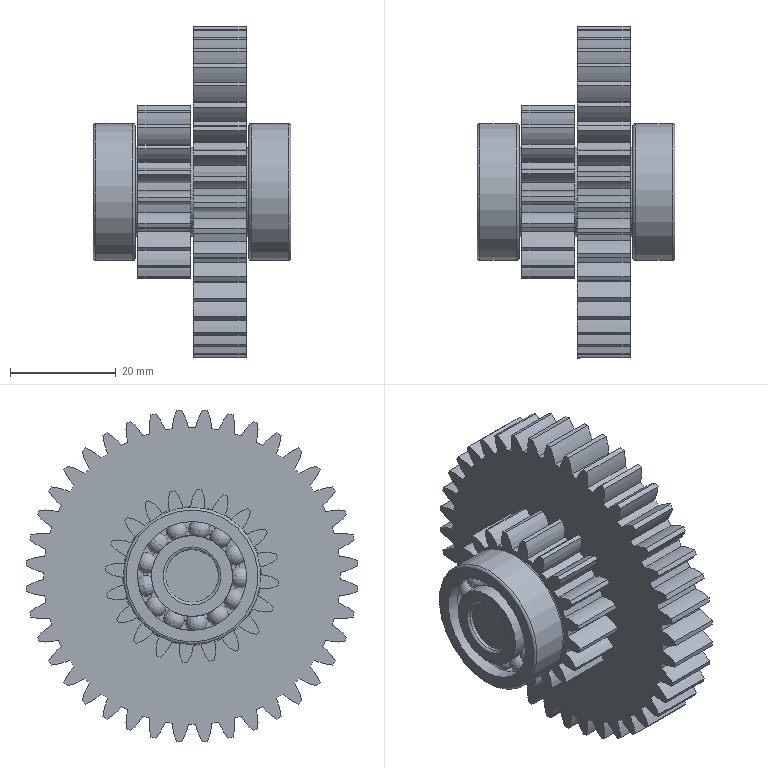Part | NX | features BREP 6 | 10 solids | 397 faces | box 37.5 x 62.872 x 62.872 mm | volume 41891 mm3 | cylinder 269 | torus 60 | plane 40 | sphere 26 | cone 2 | commonest cylinder face diameters 24 x80 12 x43 56.248 x40 63 x40 26.248 x20 33 x20